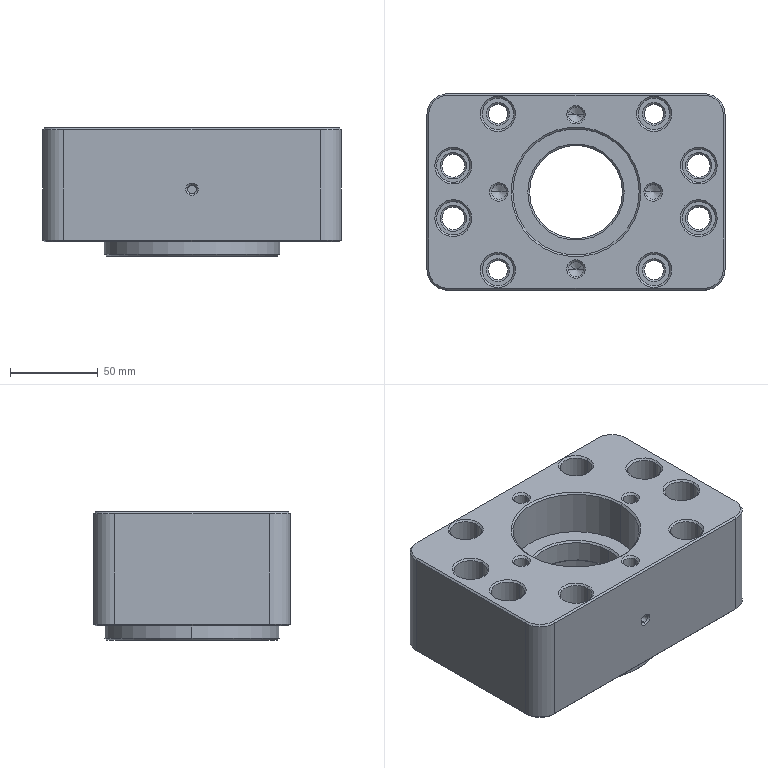NC program | NX | posted with a generic post | part box 170 x 112 x 73 mm
Lines 2627 to 2869 of 12198:
(HOLE_MILLING_COPY_1 , TOOL : D10JING)
N5216 T09 M6
N5218 G54
N5220 G17 G0 G90 X-70. Y15. S5000 M3
N5222 G43 Z30. H9
N5224 Z0.5
N5226 G94 G1 X-69.111 Y13.804 F1000.
N5228 G3 X-65.5 Y15. R2.003
N5230 X-65.5 Y15. Z-1.5 I-4.5 J0. F1200.
N5232 X-65.5 Y15. Z-3.5 I-4.5 J0.
N5234 X-65.5 Y15. Z-5.5 I-4.5 J0.
N5236 X-65.5 Y15. Z-7.5 I-4.5 J0.
N5238 X-65.5 Y15. Z-9.5 I-4.5 J0.
N5240 X-65.5 Y15. Z-11.5 I-4.5 J0.
N5242 X-65.5 Y15. Z-13.5 I-4.5 J0.
N5244 X-65.5 Y15. Z-15.5 I-4.5 J0.
N5246 X-65.5 Y15. Z-17.5 I-4.5 J0.
N5248 X-65.5 Y15. Z-19.5 I-4.5 J0.
N5250 X-65.5 Y15. Z-21.5 I-4.5 J0.
N5252 X-65.5 Y15. Z-23.5 I-4.5 J0.
N5254 X-65.5 Y15. Z-25.5 I-4.5 J0.
N5256 X-65.5 Y15. Z-27.5 I-4.5 J0.
N5258 X-65.5 Y15. Z-29.5 I-4.5 J0.
N5260 X-65.5 Y15. Z-31.5 I-4.5 J0.
N5262 X-65.5 Y15. Z-33.5 I-4.5 J0.
N5264 X-70. Y10.5 Z-35. R-4.5
N5266 X-65.5 Y15. R4.5
N5268 X-70. Y10.5 R-4.5
N5270 X-68.804 Y14.111 R2.003
N5272 G1 X-70. Y15.
N5274 G0 Z30.
N5276 X-44.5 Y44.5
N5278 Z0.5
N5280 G1 X-44.038 Y43.624 F1000.
N5282 G3 X-40.5 Y44.5 R1.877
N5284 X-40.5 Y44.5 Z-1.5 I-4. J0. F1200.
N5286 X-40.5 Y44.5 Z-3.5 I-4. J0.
N5288 X-40.5 Y44.5 Z-5.5 I-4. J0.
N5290 X-40.5 Y44.5 Z-7.5 I-4. J0.
N5292 X-40.5 Y44.5 Z-9.5 I-4. J0.
N5294 X-40.5 Y44.5 Z-11.5 I-4. J0.
N5296 X-40.5 Y44.5 Z-13.5 I-4. J0.
N5298 X-40.5 Y44.5 Z-15.5 I-4. J0.
N5300 X-40.5 Y44.5 Z-17.5 I-4. J0.
N5302 X-40.5 Y44.5 Z-19.5 I-4. J0.
N5304 X-40.5 Y44.5 Z-21.5 I-4. J0.
N5306 X-40.5 Y44.5 Z-23.5 I-4. J0.
N5308 X-40.5 Y44.5 Z-25.5 I-4. J0.
N5310 X-40.5 Y44.5 Z-27.5 I-4. J0.
N5312 X-40.5 Y44.5 Z-29.5 I-4. J0.
N5314 X-40.5 Y44.5 Z-31.5 I-4. J0.
N5316 X-40.5 Y44.5 Z-33.5 I-4. J0.
N5318 X-44.5 Y40.5 Z-35. R-4.
N5320 X-40.5 Y44.5 R4.
N5322 X-44.5 Y40.5 R-4.
N5324 X-43.624 Y44.038 R1.877
N5326 G1 X-44.5 Y44.5
N5328 G0 Z30.
N5330 X-70. Y-15.
N5332 Z0.5
N5334 G1 X-69.111 Y-16.196 F1000.
N5336 G3 X-65.5 Y-15. R2.003
N5338 X-65.5 Y-15. Z-1.5 I-4.5 J0. F1200.
N5340 X-65.5 Y-15. Z-3.5 I-4.5 J0.
N5342 X-65.5 Y-15. Z-5.5 I-4.5 J0.
N5344 X-65.5 Y-15. Z-7.5 I-4.5 J0.
N5346 X-65.5 Y-15. Z-9.5 I-4.5 J0.
N5348 X-65.5 Y-15. Z-11.5 I-4.5 J0.
N5350 X-65.5 Y-15. Z-13.5 I-4.5 J0.
N5352 X-65.5 Y-15. Z-15.5 I-4.5 J0.
N5354 X-65.5 Y-15. Z-17.5 I-4.5 J0.
N5356 X-65.5 Y-15. Z-19.5 I-4.5 J0.
N5358 X-65.5 Y-15. Z-21.5 I-4.5 J0.
N5360 X-65.5 Y-15. Z-23.5 I-4.5 J0.
N5362 X-65.5 Y-15. Z-25.5 I-4.5 J0.
N5364 X-65.5 Y-15. Z-27.5 I-4.5 J0.
N5366 X-65.5 Y-15. Z-29.5 I-4.5 J0.
N5368 X-65.5 Y-15. Z-31.5 I-4.5 J0.
N5370 X-65.5 Y-15. Z-33.5 I-4.5 J0.
N5372 X-70. Y-19.5 Z-35. R-4.5
N5374 X-65.5 Y-15. R4.5
N5376 X-70. Y-19.5 R-4.5
N5378 X-68.804 Y-15.889 R2.003
N5380 G1 X-70. Y-15.
N5382 G0 Z30.
N5384 X-44.5 Y-44.5
N5386 Z0.5
N5388 G1 X-44.038 Y-45.376 F1000.
N5390 G3 X-40.5 Y-44.5 R1.877
N5392 X-40.5 Y-44.5 Z-1.5 I-4. J0. F1200.
N5394 X-40.5 Y-44.5 Z-3.5 I-4. J0.
N5396 X-40.5 Y-44.5 Z-5.5 I-4. J0.
N5398 X-40.5 Y-44.5 Z-7.5 I-4. J0.
N5400 X-40.5 Y-44.5 Z-9.5 I-4. J0.
N5402 X-40.5 Y-44.5 Z-11.5 I-4. J0.
N5404 X-40.5 Y-44.5 Z-13.5 I-4. J0.
N5406 X-40.5 Y-44.5 Z-15.5 I-4. J0.
N5408 X-40.5 Y-44.5 Z-17.5 I-4. J0.
N5410 X-40.5 Y-44.5 Z-19.5 I-4. J0.
N5412 X-40.5 Y-44.5 Z-21.5 I-4. J0.
N5414 X-40.5 Y-44.5 Z-23.5 I-4. J0.
N5416 X-40.5 Y-44.5 Z-25.5 I-4. J0.
N5418 X-40.5 Y-44.5 Z-27.5 I-4. J0.
N5420 X-40.5 Y-44.5 Z-29.5 I-4. J0.
N5422 X-40.5 Y-44.5 Z-31.5 I-4. J0.
N5424 X-40.5 Y-44.5 Z-33.5 I-4. J0.
N5426 X-44.5 Y-48.5 Z-35. R-4.
N5428 X-40.5 Y-44.5 R4.
N5430 X-44.5 Y-48.5 R-4.
N5432 X-43.624 Y-44.962 R1.877
N5434 G1 X-44.5 Y-44.5
N5436 G0 Z30.
N5438 X44.5
N5440 Z0.5
N5442 G1 X44.962 Y-45.376 F1000.
N5444 G3 X48.5 Y-44.5 R1.877
N5446 X48.5 Y-44.5 Z-1.5 I-4. J0. F1200.
N5448 X48.5 Y-44.5 Z-3.5 I-4. J0.
N5450 X48.5 Y-44.5 Z-5.5 I-4. J0.
N5452 X48.5 Y-44.5 Z-7.5 I-4. J0.
N5454 X48.5 Y-44.5 Z-9.5 I-4. J0.
N5456 X48.5 Y-44.5 Z-11.5 I-4. J0.
N5458 X48.5 Y-44.5 Z-13.5 I-4. J0.
N5460 X48.5 Y-44.5 Z-15.5 I-4. J0.
N5462 X48.5 Y-44.5 Z-17.5 I-4. J0.
N5464 X48.5 Y-44.5 Z-19.5 I-4. J0.
N5466 X48.5 Y-44.5 Z-21.5 I-4. J0.
N5468 X48.5 Y-44.5 Z-23.5 I-4. J0.
N5470 X48.5 Y-44.5 Z-25.5 I-4. J0.
N5472 X48.5 Y-44.5 Z-27.5 I-4. J0.
N5474 X48.5 Y-44.5 Z-29.5 I-4. J0.
N5476 X48.5 Y-44.5 Z-31.5 I-4. J0.
N5478 X48.5 Y-44.5 Z-33.5 I-4. J0.
N5480 X44.5 Y-48.5 Z-35. R-4.
N5482 X48.5 Y-44.5 R4.
N5484 X44.5 Y-48.5 R-4.
N5486 X45.376 Y-44.962 R1.877
N5488 G1 X44.5 Y-44.5
N5490 G0 Z30.
N5492 X70. Y-15.
N5494 Z0.5
N5496 G1 X70.889 Y-16.196 F1000.
N5498 G3 X74.5 Y-15. R2.003
N5500 X74.5 Y-15. Z-1.5 I-4.5 J0. F1200.
N5502 X74.5 Y-15. Z-3.5 I-4.5 J0.
N5504 X74.5 Y-15. Z-5.5 I-4.5 J0.
N5506 X74.5 Y-15. Z-7.5 I-4.5 J0.
N5508 X74.5 Y-15. Z-9.5 I-4.5 J0.
N5510 X74.5 Y-15. Z-11.5 I-4.5 J0.
N5512 X74.5 Y-15. Z-13.5 I-4.5 J0.
N5514 X74.5 Y-15. Z-15.5 I-4.5 J0.
N5516 X74.5 Y-15. Z-17.5 I-4.5 J0.
N5518 X74.5 Y-15. Z-19.5 I-4.5 J0.
N5520 X74.5 Y-15. Z-21.5 I-4.5 J0.
N5522 X74.5 Y-15. Z-23.5 I-4.5 J0.
N5524 X74.5 Y-15. Z-25.5 I-4.5 J0.
N5526 X74.5 Y-15. Z-27.5 I-4.5 J0.
N5528 X74.5 Y-15. Z-29.5 I-4.5 J0.
N5530 X74.5 Y-15. Z-31.5 I-4.5 J0.
N5532 X74.5 Y-15. Z-33.5 I-4.5 J0.
N5534 X70. Y-19.5 Z-35. R-4.5
N5536 X74.5 Y-15. R4.5
N5538 X70. Y-19.5 R-4.5
N5540 X71.196 Y-15.889 R2.003
N5542 G1 X70. Y-15.
N5544 G0 Z30.
N5546 Y15.
N5548 Z0.5
N5550 G1 X70.889 Y13.804 F1000.
N5552 G3 X74.5 Y15. R2.003
N5554 X74.5 Y15. Z-1.5 I-4.5 J0. F1200.
N5556 X74.5 Y15. Z-3.5 I-4.5 J0.
N5558 X74.5 Y15. Z-5.5 I-4.5 J0.
N5560 X74.5 Y15. Z-7.5 I-4.5 J0.
N5562 X74.5 Y15. Z-9.5 I-4.5 J0.
N5564 X74.5 Y15. Z-11.5 I-4.5 J0.
N5566 X74.5 Y15. Z-13.5 I-4.5 J0.
N5568 X74.5 Y15. Z-15.5 I-4.5 J0.
N5570 X74.5 Y15. Z-17.5 I-4.5 J0.
N5572 X74.5 Y15. Z-19.5 I-4.5 J0.
N5574 X74.5 Y15. Z-21.5 I-4.5 J0.
N5576 X74.5 Y15. Z-23.5 I-4.5 J0.
N5578 X74.5 Y15. Z-25.5 I-4.5 J0.
N5580 X74.5 Y15. Z-27.5 I-4.5 J0.
N5582 X74.5 Y15. Z-29.5 I-4.5 J0.
N5584 X74.5 Y15. Z-31.5 I-4.5 J0.
N5586 X74.5 Y15. Z-33.5 I-4.5 J0.
N5588 X70. Y10.5 Z-35. R-4.5
N5590 X74.5 Y15. R4.5
N5592 X70. Y10.5 R-4.5
N5594 X71.196 Y14.111 R2.003
N5596 G1 X70. Y15.
N5598 G0 Z30.
N5600 X44.5 Y44.5
N5602 Z0.5
N5604 G1 X44.962 Y43.624 F1000.
N5606 G3 X48.5 Y44.5 R1.877
N5608 X48.5 Y44.5 Z-1.5 I-4. J0. F1200.
N5610 X48.5 Y44.5 Z-3.5 I-4. J0.
N5612 X48.5 Y44.5 Z-5.5 I-4. J0.
N5614 X48.5 Y44.5 Z-7.5 I-4. J0.
N5616 X48.5 Y44.5 Z-9.5 I-4. J0.
N5618 X48.5 Y44.5 Z-11.5 I-4. J0.
N5620 X48.5 Y44.5 Z-13.5 I-4. J0.
N5622 X48.5 Y44.5 Z-15.5 I-4. J0.
N5624 X48.5 Y44.5 Z-17.5 I-4. J0.
N5626 X48.5 Y44.5 Z-19.5 I-4. J0.
N5628 X48.5 Y44.5 Z-21.5 I-4. J0.
N5630 X48.5 Y44.5 Z-23.5 I-4. J0.
N5632 X48.5 Y44.5 Z-25.5 I-4. J0.
N5634 X48.5 Y44.5 Z-27.5 I-4. J0.
N5636 X48.5 Y44.5 Z-29.5 I-4. J0.
N5638 X48.5 Y44.5 Z-31.5 I-4. J0.
N5640 X48.5 Y44.5 Z-33.5 I-4. J0.
N5642 X44.5 Y40.5 Z-35. R-4.
N5644 X48.5 Y44.5 R4.
N5646 X44.5 Y40.5 R-4.
N5648 X45.376 Y44.038 R1.877
N5650 G1 X44.5 Y44.5
N5652 G0 Z30.
(HOLE_MILLING_COPY_1_COPY , TOOL : D10JING)
N5654 X0. Y0.
N5656 Z-26.5
N5658 G1 X17.72 Y-3.165 F1000.
N5660 G3 X21.5 Y0. R3.215
N5662 X21.5 Y0. Z-28.5 I-21.5 J0. F1200.
N5664 X21.5 Y0. Z-30.5 I-21.5 J0.
N5666 X21.5 Y0. Z-32.5 I-21.5 J0.
N5668 X21.5 Y0. Z-34.5 I-21.5 J0.
N5670 X21.5 Y0. Z-36.5 I-21.5 J0.
N5672 X21.5 Y0. Z-38.5 I-21.5 J0.
N5674 X21.5 Y0. Z-40.5 I-21.5 J0.
N5676 X0. Y21.5 Z-41. R21.5
N5678 X-21.5 Y0. R21.5
N5680 X0. Y21.5 R-21.5
N5682 X-3.165 Y17.72 R3.215
N5684 G1 X0. Y0.
N5686 G0 Z30.
N5688 M5